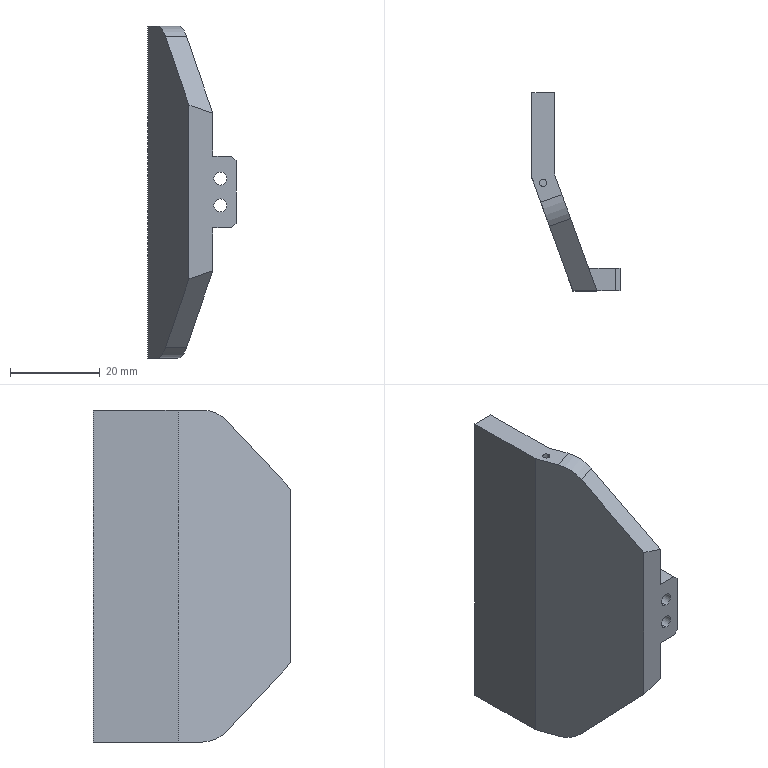Part | NX | 1 solid | 38 faces | box 19.643 x 44.061 x 74 mm | volume 15550 mm3 | plane 20 | cylinder 10 | cone 8 | commonest cylinder face diameters 1.6 x4 2.9 x4 16 x2
STEP:
#1=CARTESIAN_POINT('',(-19.643,44.061,-74.));
#2=VERTEX_POINT('',#1);
#3=CARTESIAN_POINT('',(-19.643,44.061,0.));
#4=VERTEX_POINT('',#3);
#5=CARTESIAN_POINT('',(-19.643,44.061,-74.));
#6=DIRECTION('',(0.,0.,1.));
#7=VECTOR('',#6,1000.);
#8=LINE('',#5,#7);
#9=EDGE_CURVE('',#2,#4,#8,.T.);
#10=ORIENTED_EDGE('',*,*,#9,.F.);
#11=CARTESIAN_POINT('',(-19.643,25.118,-74.));
#12=VERTEX_POINT('',#11);
#13=CARTESIAN_POINT('',(-19.643,34.6,-74.));
#14=DIRECTION('',(0.,-1.,0.));
#15=VECTOR('',#14,1000.);
#16=LINE('',#13,#15);
#17=EDGE_CURVE('',#2,#12,#16,.T.);
#18=ORIENTED_EDGE('',*,*,#17,.T.);
#19=CARTESIAN_POINT('',(-19.643,25.118,0.));
#20=VERTEX_POINT('',#19);
#21=CARTESIAN_POINT('',(-19.643,25.118,-74.));
#22=DIRECTION('',(0.,0.,1.));
#23=VECTOR('',#22,1000.);
#24=LINE('',#21,#23);
#25=EDGE_CURVE('',#12,#20,#24,.T.);
#26=ORIENTED_EDGE('',*,*,#25,.T.);
#27=CARTESIAN_POINT('',(-19.643,34.6,0.));
#28=DIRECTION('',(0.,-1.,0.));
#29=VECTOR('',#28,1000.);
#30=LINE('',#27,#29);
#31=EDGE_CURVE('',#4,#20,#30,.T.);
#32=ORIENTED_EDGE('',*,*,#31,.F.);
#33=EDGE_LOOP('',(#10,#18,#26,#32));
#34=FACE_BOUND('',#33,.T.);
#35=CARTESIAN_POINT('',(-19.643,34.6,-74.));
#36=DIRECTION('',(-1.,0.,0.));
#37=DIRECTION('',(0.,0.,1.));
#38=AXIS2_PLACEMENT_3D('',#35,#36,#37);
#39=PLANE('',#38);
#40=ADVANCED_FACE('',(#34),#39,.T.);
#41=CARTESIAN_POINT('',(-14.643,26.,0.));
#42=VERTEX_POINT('',#41);
#43=CARTESIAN_POINT('',(-14.643,44.061,0.));
#44=VERTEX_POINT('',#43);
#45=CARTESIAN_POINT('',(-14.643,34.6,0.));
#46=DIRECTION('',(0.,1.,0.));
#47=VECTOR('',#46,1000.);
#48=LINE('',#45,#47);
#49=EDGE_CURVE('',#42,#44,#48,.T.);
#50=ORIENTED_EDGE('',*,*,#49,.T.);
#51=CARTESIAN_POINT('',(0.,44.061,0.));
#52=DIRECTION('',(-1.,0.,0.));
#53=VECTOR('',#52,1000.);
#54=LINE('',#51,#53);
#55=EDGE_CURVE('',#44,#4,#54,.T.);
#56=ORIENTED_EDGE('',*,*,#55,.T.);
#57=ORIENTED_EDGE('',*,*,#31,.T.);
#58=CARTESIAN_POINT('',(-17.662,19.674,0.));
#59=VERTEX_POINT('',#58);
#60=CARTESIAN_POINT('',(-10.501,0.,0.));
#61=DIRECTION('',(0.342,-0.9397,0.));
#62=VECTOR('',#61,1000.);
#63=LINE('',#60,#62);
#64=EDGE_CURVE('',#20,#59,#63,.T.);
#65=ORIENTED_EDGE('',*,*,#64,.T.);
#66=CARTESIAN_POINT('',(-12.963,21.384,0.));
#67=VERTEX_POINT('',#66);
#68=CARTESIAN_POINT('',(-12.963,21.384,0.));
#69=DIRECTION('',(0.9397,0.342,0.));
#70=VECTOR('',#69,1000.);
#71=LINE('',#68,#70);
#72=EDGE_CURVE('',#59,#67,#71,.T.);
#73=ORIENTED_EDGE('',*,*,#72,.T.);
#74=CARTESIAN_POINT('',(-14.643,26.,0.));
#75=DIRECTION('',(-0.342,0.9397,0.));
#76=VECTOR('',#75,1000.);
#77=LINE('',#74,#76);
#78=EDGE_CURVE('',#67,#42,#77,.T.);
#79=ORIENTED_EDGE('',*,*,#78,.T.);
#80=EDGE_LOOP('',(#50,#56,#57,#65,#73,#79));
#81=FACE_BOUND('',#80,.T.);
#82=CARTESIAN_POINT('',(-17.943,24.061,0.));
#83=VERTEX_POINT('',#82);
#84=CARTESIAN_POINT('',(-16.343,24.061,0.));
#85=VERTEX_POINT('',#84);
#86=CARTESIAN_POINT('',(-17.143,24.061,0.));
#87=DIRECTION('',(0.,0.,-1.));
#88=DIRECTION('',(-1.,0.,0.));
#89=AXIS2_PLACEMENT_3D('',#86,#87,#88);
#90=CIRCLE('',#89,0.8);
#91=EDGE_CURVE('',#83,#85,#90,.T.);
#92=ORIENTED_EDGE('',*,*,#91,.T.);
#93=CARTESIAN_POINT('',(-17.143,24.061,0.));
#94=DIRECTION('',(0.,0.,-1.));
#95=DIRECTION('',(-1.,0.,0.));
#96=AXIS2_PLACEMENT_3D('',#93,#94,#95);
#97=CIRCLE('',#96,0.8);
#98=EDGE_CURVE('',#85,#83,#97,.T.);
#99=ORIENTED_EDGE('',*,*,#98,.T.);
#100=EDGE_LOOP('',(#92,#99));
#101=FACE_BOUND('',#100,.T.);
#102=CARTESIAN_POINT('',(0.,0.,0.));
#103=DIRECTION('',(0.,0.,-1.));
#104=DIRECTION('',(-1.,0.,0.));
#105=AXIS2_PLACEMENT_3D('',#102,#103,#104);
#106=PLANE('',#105);
#107=ADVANCED_FACE('',(#81,#101),#106,.F.);
#108=CARTESIAN_POINT('',(-14.643,44.061,-74.));
#109=VERTEX_POINT('',#108);
#110=CARTESIAN_POINT('',(0.,44.061,-74.));
#111=DIRECTION('',(-1.,0.,0.));
#112=VECTOR('',#111,1000.);
#113=LINE('',#110,#112);
#114=EDGE_CURVE('',#109,#2,#113,.T.);
#115=ORIENTED_EDGE('',*,*,#114,.F.);
#116=CARTESIAN_POINT('',(-14.643,26.,-74.));
#117=VERTEX_POINT('',#116);
#118=CARTESIAN_POINT('',(-14.643,34.6,-74.));
#119=DIRECTION('',(0.,1.,0.));
#120=VECTOR('',#119,1000.);
#121=LINE('',#118,#120);
#122=EDGE_CURVE('',#117,#109,#121,.T.);
#123=ORIENTED_EDGE('',*,*,#122,.F.);
#124=CARTESIAN_POINT('',(-12.963,21.384,-74.));
#125=VERTEX_POINT('',#124);
#126=CARTESIAN_POINT('',(-14.643,26.,-74.));
#127=DIRECTION('',(-0.342,0.9397,0.));
#128=VECTOR('',#127,1000.);
#129=LINE('',#126,#128);
#130=EDGE_CURVE('',#125,#117,#129,.T.);
#131=ORIENTED_EDGE('',*,*,#130,.F.);
#132=CARTESIAN_POINT('',(-17.662,19.674,-74.));
#133=VERTEX_POINT('',#132);
#134=CARTESIAN_POINT('',(-17.662,19.674,-74.));
#135=DIRECTION('',(-0.9397,-0.342,0.));
#136=VECTOR('',#135,1000.);
#137=LINE('',#134,#136);
#138=EDGE_CURVE('',#125,#133,#137,.T.);
#139=ORIENTED_EDGE('',*,*,#138,.T.);
#140=CARTESIAN_POINT('',(-10.501,0.,-74.));
#141=DIRECTION('',(0.342,-0.9397,0.));
#142=VECTOR('',#141,1000.);
#143=LINE('',#140,#142);
#144=EDGE_CURVE('',#12,#133,#143,.T.);
#145=ORIENTED_EDGE('',*,*,#144,.F.);
#146=ORIENTED_EDGE('',*,*,#17,.F.);
#147=EDGE_LOOP('',(#115,#123,#131,#139,#145,#146));
#148=FACE_BOUND('',#147,.T.);
#149=CARTESIAN_POINT('',(-17.943,24.061,-74.));
#150=VERTEX_POINT('',#149);
#151=CARTESIAN_POINT('',(-16.343,24.061,-74.));
#152=VERTEX_POINT('',#151);
#153=CARTESIAN_POINT('',(-17.143,24.061,-74.));
#154=DIRECTION('',(0.,0.,-1.));
#155=DIRECTION('',(-1.,0.,0.));
#156=AXIS2_PLACEMENT_3D('',#153,#154,#155);
#157=CIRCLE('',#156,0.8);
#158=EDGE_CURVE('',#150,#152,#157,.T.);
#159=ORIENTED_EDGE('',*,*,#158,.F.);
#160=CARTESIAN_POINT('',(-17.143,24.061,-74.));
#161=DIRECTION('',(0.,0.,-1.));
#162=DIRECTION('',(-1.,0.,0.));
#163=AXIS2_PLACEMENT_3D('',#160,#161,#162);
#164=CIRCLE('',#163,0.8);
#165=EDGE_CURVE('',#152,#150,#164,.T.);
#166=ORIENTED_EDGE('',*,*,#165,.F.);
#167=EDGE_LOOP('',(#159,#166));
#168=FACE_BOUND('',#167,.T.);
#169=CARTESIAN_POINT('',(0.,0.,-74.));
#170=DIRECTION('',(0.,0.,-1.));
#171=DIRECTION('',(-1.,0.,0.));
#172=AXIS2_PLACEMENT_3D('',#169,#170,#171);
#173=PLANE('',#172);
#174=ADVANCED_FACE('',(#148,#168),#173,.T.);
#175=CARTESIAN_POINT('',(-17.943,24.061,-5.));
#176=VERTEX_POINT('',#175);
#177=CARTESIAN_POINT('',(-17.943,24.061,-74.));
#178=DIRECTION('',(0.,0.,-1.));
#179=VECTOR('',#178,1000.);
#180=LINE('',#177,#179);
#181=EDGE_CURVE('',#176,#83,#180,.F.);
#182=ORIENTED_EDGE('',*,*,#181,.F.);
#183=CARTESIAN_POINT('',(-16.343,24.061,-5.));
#184=VERTEX_POINT('',#183);
#185=CARTESIAN_POINT('',(-17.143,24.061,-5.));
#186=DIRECTION('',(0.,0.,1.));
#187=DIRECTION('',(1.,0.,0.));
#188=AXIS2_PLACEMENT_3D('',#185,#186,#187);
#189=CIRCLE('',#188,0.8);
#190=EDGE_CURVE('',#176,#184,#189,.F.);
#191=ORIENTED_EDGE('',*,*,#190,.T.);
#192=CARTESIAN_POINT('',(-16.343,24.061,-74.));
#193=DIRECTION('',(0.,0.,-1.));
#194=VECTOR('',#193,1000.);
#195=LINE('',#192,#194);
#196=EDGE_CURVE('',#184,#85,#195,.F.);
#197=ORIENTED_EDGE('',*,*,#196,.T.);
#198=ORIENTED_EDGE('',*,*,#91,.F.);
#199=EDGE_LOOP('',(#182,#191,#197,#198));
#200=FACE_BOUND('',#199,.T.);
#201=CARTESIAN_POINT('',(-17.143,24.061,-74.));
#202=DIRECTION('',(0.,0.,-1.));
#203=DIRECTION('',(-1.,0.,0.));
#204=AXIS2_PLACEMENT_3D('',#201,#202,#203);
#205=CYLINDRICAL_SURFACE('',#204,0.8);
#206=ADVANCED_FACE('',(#200),#205,.F.);
#207=CARTESIAN_POINT('',(-16.343,24.061,-68.));
#208=VERTEX_POINT('',#207);
#209=CARTESIAN_POINT('',(-16.343,24.061,-74.));
#210=DIRECTION('',(0.,0.,-1.));
#211=VECTOR('',#210,1000.);
#212=LINE('',#209,#211);
#213=EDGE_CURVE('',#152,#208,#212,.F.);
#214=ORIENTED_EDGE('',*,*,#213,.T.);
#215=CARTESIAN_POINT('',(-17.943,24.061,-68.));
#216=VERTEX_POINT('',#215);
#217=CARTESIAN_POINT('',(-17.143,24.061,-68.));
#218=DIRECTION('',(0.,0.,1.));
#219=DIRECTION('',(1.,0.,0.));
#220=AXIS2_PLACEMENT_3D('',#217,#218,#219);
#221=CIRCLE('',#220,0.8);
#222=EDGE_CURVE('',#208,#216,#221,.T.);
#223=ORIENTED_EDGE('',*,*,#222,.T.);
#224=CARTESIAN_POINT('',(-17.943,24.061,-74.));
#225=DIRECTION('',(0.,0.,-1.));
#226=VECTOR('',#225,1000.);
#227=LINE('',#224,#226);
#228=EDGE_CURVE('',#150,#216,#227,.F.);
#229=ORIENTED_EDGE('',*,*,#228,.F.);
#230=ORIENTED_EDGE('',*,*,#158,.T.);
#231=EDGE_LOOP('',(#214,#223,#229,#230));
#232=FACE_BOUND('',#231,.T.);
#233=CARTESIAN_POINT('',(-17.143,24.061,-74.));
#234=DIRECTION('',(0.,0.,-1.));
#235=DIRECTION('',(-1.,0.,0.));
#236=AXIS2_PLACEMENT_3D('',#233,#234,#235);
#237=CYLINDRICAL_SURFACE('',#236,0.8);
#238=ADVANCED_FACE('',(#232),#237,.F.);
#239=CARTESIAN_POINT('',(0.,0.,-30.));
#240=VERTEX_POINT('',#239);
#241=CARTESIAN_POINT('',(-1.,0.,-29.));
#242=VERTEX_POINT('',#241);
#243=CARTESIAN_POINT('',(22.,0.,-52.));
#244=DIRECTION('',(-0.7071,0.,0.7071));
#245=VECTOR('',#244,1000.);
#246=LINE('',#243,#245);
#247=EDGE_CURVE('',#240,#242,#246,.T.);
#248=ORIENTED_EDGE('',*,*,#247,.F.);
#249=CARTESIAN_POINT('',(0.,5.,-30.));
#250=VERTEX_POINT('',#249);
#251=CARTESIAN_POINT('',(0.,5.,-30.));
#252=DIRECTION('',(0.,-1.,0.));
#253=VECTOR('',#252,1000.);
#254=LINE('',#251,#253);
#255=EDGE_CURVE('',#250,#240,#254,.T.);
#256=ORIENTED_EDGE('',*,*,#255,.F.);
#257=CARTESIAN_POINT('',(-1.,5.,-29.));
#258=VERTEX_POINT('',#257);
#259=CARTESIAN_POINT('',(18.5,5.,-48.5));
#260=DIRECTION('',(0.7071,0.,-0.7071));
#261=VECTOR('',#260,1000.);
#262=LINE('',#259,#261);
#263=EDGE_CURVE('',#258,#250,#262,.T.);
#264=ORIENTED_EDGE('',*,*,#263,.F.);
#265=CARTESIAN_POINT('',(-1.,4.336,-29.));
#266=DIRECTION('',(0.,1.,0.));
#267=VECTOR('',#266,1000.);
#268=LINE('',#265,#267);
#269=EDGE_CURVE('',#242,#258,#268,.T.);
#270=ORIENTED_EDGE('',*,*,#269,.F.);
#271=EDGE_LOOP('',(#248,#256,#264,#270));
#272=FACE_BOUND('',#271,.T.);
#273=CARTESIAN_POINT('',(-1.,4.336,-29.));
#274=DIRECTION('',(-0.7071,0.,-0.7071));
#275=DIRECTION('',(0.,1.,0.));
#276=AXIS2_PLACEMENT_3D('',#273,#274,#275);
#277=PLANE('',#276);
#278=ADVANCED_FACE('',(#272),#277,.F.);
#279=CARTESIAN_POINT('',(0.,5.,-44.));
#280=VERTEX_POINT('',#279);
#281=CARTESIAN_POINT('',(-1.,5.,-45.));
#282=VERTEX_POINT('',#281);
#283=CARTESIAN_POINT('',(-18.5,5.,-62.5));
#284=DIRECTION('',(-0.7071,0.,-0.7071));
#285=VECTOR('',#284,1000.);
#286=LINE('',#283,#285);
#287=EDGE_CURVE('',#280,#282,#286,.T.);
#288=ORIENTED_EDGE('',*,*,#287,.F.);
#289=CARTESIAN_POINT('',(0.,0.,-44.));
#290=VERTEX_POINT('',#289);
#291=CARTESIAN_POINT('',(0.,5.,-44.));
#292=DIRECTION('',(0.,1.,0.));
#293=VECTOR('',#292,1000.);
#294=LINE('',#291,#293);
#295=EDGE_CURVE('',#290,#280,#294,.T.);
#296=ORIENTED_EDGE('',*,*,#295,.F.);
#297=CARTESIAN_POINT('',(-1.,0.,-45.));
#298=VERTEX_POINT('',#297);
#299=CARTESIAN_POINT('',(-15.,0.,-59.));
#300=DIRECTION('',(0.7071,0.,0.7071));
#301=VECTOR('',#300,1000.);
#302=LINE('',#299,#301);
#303=EDGE_CURVE('',#298,#290,#302,.T.);
#304=ORIENTED_EDGE('',*,*,#303,.F.);
#305=CARTESIAN_POINT('',(-1.,18.819,-45.));
#306=DIRECTION('',(0.,-1.,0.));
#307=VECTOR('',#306,1000.);
#308=LINE('',#305,#307);
#309=EDGE_CURVE('',#282,#298,#308,.T.);
#310=ORIENTED_EDGE('',*,*,#309,.F.);
#311=EDGE_LOOP('',(#288,#296,#304,#310));
#312=FACE_BOUND('',#311,.T.);
#313=CARTESIAN_POINT('',(-1.,18.819,-45.));
#314=DIRECTION('',(-0.7071,0.,0.7071));
#315=DIRECTION('',(0.,-1.,0.));
#316=AXIS2_PLACEMENT_3D('',#313,#314,#315);
#317=PLANE('',#316);
#318=ADVANCED_FACE('',(#312),#317,.F.);
#319=CARTESIAN_POINT('',(-3.5,3.7,-35.45));
#320=VERTEX_POINT('',#319);
#321=CARTESIAN_POINT('',(-3.5,5.,-36.75));
#322=VERTEX_POINT('',#321);
#323=CARTESIAN_POINT('',(-3.5,5.,-36.75));
#324=DIRECTION('',(0.,0.7071,-0.7071));
#325=VECTOR('',#324,1000.);
#326=LINE('',#323,#325);
#327=EDGE_CURVE('',#320,#322,#326,.T.);
#328=ORIENTED_EDGE('',*,*,#327,.F.);
#329=CARTESIAN_POINT('',(-3.5,3.7,-32.55));
#330=VERTEX_POINT('',#329);
#331=CARTESIAN_POINT('',(-3.5,3.7,-34.));
#332=DIRECTION('',(0.,1.,0.));
#333=DIRECTION('',(0.,0.,1.));
#334=AXIS2_PLACEMENT_3D('',#331,#332,#333);
#335=CIRCLE('',#334,1.45);
#336=EDGE_CURVE('',#330,#320,#335,.T.);
#337=ORIENTED_EDGE('',*,*,#336,.F.);
#338=CARTESIAN_POINT('',(-3.5,5.,-31.25));
#339=VERTEX_POINT('',#338);
#340=CARTESIAN_POINT('',(-3.5,5.,-31.25));
#341=DIRECTION('',(0.,0.7071,0.7071));
#342=VECTOR('',#341,1000.);
#343=LINE('',#340,#342);
#344=EDGE_CURVE('',#330,#339,#343,.T.);
#345=ORIENTED_EDGE('',*,*,#344,.T.);
#346=CARTESIAN_POINT('',(-3.5,5.,-34.));
#347=DIRECTION('',(0.,1.,0.));
#348=DIRECTION('',(0.,0.,1.));
#349=AXIS2_PLACEMENT_3D('',#346,#347,#348);
#350=CIRCLE('',#349,2.75);
#351=EDGE_CURVE('',#339,#322,#350,.T.);
#352=ORIENTED_EDGE('',*,*,#351,.T.);
#353=EDGE_LOOP('',(#328,#337,#345,#352));
#354=FACE_BOUND('',#353,.T.);
#355=CARTESIAN_POINT('',(-3.5,5.,-34.));
#356=DIRECTION('',(0.,1.,0.));
#357=DIRECTION('',(0.,0.,1.));
#358=AXIS2_PLACEMENT_3D('',#355,#356,#357);
#359=CONICAL_SURFACE('',#358,2.75,0.7854);
#360=ADVANCED_FACE('',(#354),#359,.F.);
#361=CARTESIAN_POINT('',(-3.5,0.,-35.45));
#362=VERTEX_POINT('',#361);
#363=CARTESIAN_POINT('',(-3.5,5.,-35.45));
#364=DIRECTION('',(0.,1.,0.));
#365=VECTOR('',#364,1000.);
#366=LINE('',#363,#365);
#367=EDGE_CURVE('',#362,#320,#366,.T.);
#368=ORIENTED_EDGE('',*,*,#367,.F.);
#369=CARTESIAN_POINT('',(-3.5,0.,-32.55));
#370=VERTEX_POINT('',#369);
#371=CARTESIAN_POINT('',(-3.5,0.,-34.));
#372=DIRECTION('',(0.,-1.,0.));
#373=DIRECTION('',(1.,0.,0.));
#374=AXIS2_PLACEMENT_3D('',#371,#372,#373);
#375=CIRCLE('',#374,1.45);
#376=EDGE_CURVE('',#362,#370,#375,.T.);
#377=ORIENTED_EDGE('',*,*,#376,.T.);
#378=CARTESIAN_POINT('',(-3.5,5.,-32.55));
#379=DIRECTION('',(0.,1.,0.));
#380=VECTOR('',#379,1000.);
#381=LINE('',#378,#380);
#382=EDGE_CURVE('',#370,#330,#381,.T.);
#383=ORIENTED_EDGE('',*,*,#382,.T.);
#384=ORIENTED_EDGE('',*,*,#336,.T.);
#385=EDGE_LOOP('',(#368,#377,#383,#384));
#386=FACE_BOUND('',#385,.T.);
#387=CARTESIAN_POINT('',(-3.5,5.,-34.));
#388=DIRECTION('',(0.,1.,0.));
#389=DIRECTION('',(0.,0.,1.));
#390=AXIS2_PLACEMENT_3D('',#387,#388,#389);
#391=CYLINDRICAL_SURFACE('',#390,1.45);
#392=ADVANCED_FACE('',(#386),#391,.F.);
#393=CARTESIAN_POINT('',(-3.5,3.7,-41.45));
#394=VERTEX_POINT('',#393);
#395=CARTESIAN_POINT('',(-3.5,5.,-42.75));
#396=VERTEX_POINT('',#395);
#397=CARTESIAN_POINT('',(-3.5,5.,-42.75));
#398=DIRECTION('',(0.,0.7071,-0.7071));
#399=VECTOR('',#398,1000.);
#400=LINE('',#397,#399);
#401=EDGE_CURVE('',#394,#396,#400,.T.);
#402=ORIENTED_EDGE('',*,*,#401,.F.);
#403=CARTESIAN_POINT('',(-3.5,3.7,-38.55));
#404=VERTEX_POINT('',#403);
#405=CARTESIAN_POINT('',(-3.5,3.7,-40.));
#406=DIRECTION('',(0.,1.,0.));
#407=DIRECTION('',(0.,0.,1.));
#408=AXIS2_PLACEMENT_3D('',#405,#406,#407);
#409=CIRCLE('',#408,1.45);
#410=EDGE_CURVE('',#404,#394,#409,.T.);
#411=ORIENTED_EDGE('',*,*,#410,.F.);
#412=CARTESIAN_POINT('',(-3.5,5.,-37.25));
#413=VERTEX_POINT('',#412);
#414=CARTESIAN_POINT('',(-3.5,5.,-37.25));
#415=DIRECTION('',(0.,0.7071,0.7071));
#416=VECTOR('',#415,1000.);
#417=LINE('',#414,#416);
#418=EDGE_CURVE('',#404,#413,#417,.T.);
#419=ORIENTED_EDGE('',*,*,#418,.T.);
#420=CARTESIAN_POINT('',(-3.5,5.,-40.));
#421=DIRECTION('',(0.,1.,0.));
#422=DIRECTION('',(0.,0.,1.));
#423=AXIS2_PLACEMENT_3D('',#420,#421,#422);
#424=CIRCLE('',#423,2.75);
#425=EDGE_CURVE('',#413,#396,#424,.T.);
#426=ORIENTED_EDGE('',*,*,#425,.T.);
#427=EDGE_LOOP('',(#402,#411,#419,#426));
#428=FACE_BOUND('',#427,.T.);
#429=CARTESIAN_POINT('',(-3.5,5.,-40.));
#430=DIRECTION('',(0.,1.,0.));
#431=DIRECTION('',(0.,0.,1.));
#432=AXIS2_PLACEMENT_3D('',#429,#430,#431);
#433=CONICAL_SURFACE('',#432,2.75,0.7854);
#434=ADVANCED_FACE('',(#428),#433,.F.);
#435=CARTESIAN_POINT('',(-3.5,0.,-41.45));
#436=VERTEX_POINT('',#435);
#437=CARTESIAN_POINT('',(-3.5,5.,-41.45));
#438=DIRECTION('',(0.,1.,0.));
#439=VECTOR('',#438,1000.);
#440=LINE('',#437,#439);
#441=EDGE_CURVE('',#436,#394,#440,.T.);
#442=ORIENTED_EDGE('',*,*,#441,.F.);
#443=CARTESIAN_POINT('',(-3.5,0.,-38.55));
#444=VERTEX_POINT('',#443);
#445=CARTESIAN_POINT('',(-3.5,0.,-40.));
#446=DIRECTION('',(0.,-1.,0.));
#447=DIRECTION('',(1.,0.,0.));
#448=AXIS2_PLACEMENT_3D('',#445,#446,#447);
#449=CIRCLE('',#448,1.45);
#450=EDGE_CURVE('',#436,#444,#449,.T.);
#451=ORIENTED_EDGE('',*,*,#450,.T.);
#452=CARTESIAN_POINT('',(-3.5,5.,-38.55));
#453=DIRECTION('',(0.,1.,0.));
#454=VECTOR('',#453,1000.);
#455=LINE('',#452,#454);
#456=EDGE_CURVE('',#444,#404,#455,.T.);
#457=ORIENTED_EDGE('',*,*,#456,.T.);
#458=ORIENTED_EDGE('',*,*,#410,.T.);
#459=EDGE_LOOP('',(#442,#451,#457,#458));
#460=FACE_BOUND('',#459,.T.);
#461=CARTESIAN_POINT('',(-3.5,5.,-40.));
#462=DIRECTION('',(0.,1.,0.));
#463=DIRECTION('',(0.,0.,1.));
#464=AXIS2_PLACEMENT_3D('',#461,#462,#463);
#465=CYLINDRICAL_SURFACE('',#464,1.45);
#466=ADVANCED_FACE('',(#460),#465,.F.);
#467=CARTESIAN_POINT('',(-7.,5.,-45.));
#468=VERTEX_POINT('',#467);
#469=CARTESIAN_POINT('',(6.641,5.,-45.));
#470=DIRECTION('',(1.,0.,0.));
#471=VECTOR('',#470,1000.);
#472=LINE('',#469,#471);
#473=EDGE_CURVE('',#468,#282,#472,.T.);
#474=ORIENTED_EDGE('',*,*,#473,.T.);
#475=ORIENTED_EDGE('',*,*,#309,.T.);
#476=CARTESIAN_POINT('',(-5.18,0.,-45.));
#477=VERTEX_POINT('',#476);
#478=CARTESIAN_POINT('',(6.641,0.,-45.));
#479=DIRECTION('',(-1.,0.,0.));
#480=VECTOR('',#479,1000.);
#481=LINE('',#478,#480);
#482=EDGE_CURVE('',#298,#477,#481,.T.);
#483=ORIENTED_EDGE('',*,*,#482,.T.);
#484=CARTESIAN_POINT('',(-9.846,12.819,-45.));
#485=DIRECTION('',(0.342,-0.9397,0.));
#486=VECTOR('',#485,1000.);
#487=LINE('',#484,#486);
#488=EDGE_CURVE('',#468,#477,#487,.T.);
#489=ORIENTED_EDGE('',*,*,#488,.F.);
#490=EDGE_LOOP('',(#474,#475,#483,#489));
#491=FACE_BOUND('',#490,.T.);
#492=CARTESIAN_POINT('',(6.641,18.819,-45.));
#493=DIRECTION('',(0.,0.,-1.));
#494=DIRECTION('',(-1.,0.,0.));
#495=AXIS2_PLACEMENT_3D('',#492,#493,#494);
#496=PLANE('',#495);
#497=ADVANCED_FACE('',(#491),#496,.T.);
#498=CARTESIAN_POINT('',(-5.18,0.,-29.));
#499=VERTEX_POINT('',#498);
#500=CARTESIAN_POINT('',(11.912,0.,-29.));
#501=DIRECTION('',(1.,0.,0.));
#502=VECTOR('',#501,1000.);
#503=LINE('',#500,#502);
#504=EDGE_CURVE('',#499,#242,#503,.T.);
#505=ORIENTED_EDGE('',*,*,#504,.T.);
#506=ORIENTED_EDGE('',*,*,#269,.T.);
#507=CARTESIAN_POINT('',(-7.,5.,-29.));
#508=VERTEX_POINT('',#507);
#509=CARTESIAN_POINT('',(11.912,5.,-29.));
#510=DIRECTION('',(-1.,0.,0.));
#511=VECTOR('',#510,1000.);
#512=LINE('',#509,#511);
#513=EDGE_CURVE('',#258,#508,#512,.T.);
#514=ORIENTED_EDGE('',*,*,#513,.T.);
#515=CARTESIAN_POINT('',(-4.574,-1.665,-29.));
#516=DIRECTION('',(-0.342,0.9397,0.));
#517=VECTOR('',#516,1000.);
#518=LINE('',#515,#517);
#519=EDGE_CURVE('',#499,#508,#518,.T.);
#520=ORIENTED_EDGE('',*,*,#519,.F.);
#521=EDGE_LOOP('',(#505,#506,#514,#520));
#522=FACE_BOUND('',#521,.T.);
#523=CARTESIAN_POINT('',(11.912,4.336,-29.));
#524=DIRECTION('',(0.,0.,1.));
#525=DIRECTION('',(1.,0.,0.));
#526=AXIS2_PLACEMENT_3D('',#523,#524,#525);
#527=PLANE('',#526);
#528=ADVANCED_FACE('',(#522),#527,.T.);
#529=CARTESIAN_POINT('',(-15.727,14.359,-71.657));
#530=VERTEX_POINT('',#529);
#531=CARTESIAN_POINT('',(-17.662,19.674,-66.));
#532=DIRECTION('',(-0.9397,-0.342,0.));
#533=DIRECTION('',(0.342,-0.9397,0.));
#534=AXIS2_PLACEMENT_3D('',#531,#532,#533);
#535=CIRCLE('',#534,8.);
#536=EDGE_CURVE('',#133,#530,#535,.T.);
#537=ORIENTED_EDGE('',*,*,#536,.F.);
#538=ORIENTED_EDGE('',*,*,#138,.F.);
#539=CARTESIAN_POINT('',(-11.029,16.069,-71.657));
#540=VERTEX_POINT('',#539);
#541=CARTESIAN_POINT('',(-12.963,21.384,-66.));
#542=DIRECTION('',(0.9397,0.342,0.));
#543=DIRECTION('',(-0.342,0.9397,0.));
#544=AXIS2_PLACEMENT_3D('',#541,#542,#543);
#545=CIRCLE('',#544,8.);
#546=EDGE_CURVE('',#540,#125,#545,.T.);
#547=ORIENTED_EDGE('',*,*,#546,.F.);
#548=CARTESIAN_POINT('',(-11.029,16.069,-71.657));
#549=DIRECTION('',(0.9397,0.342,0.));
#550=VECTOR('',#549,1000.);
#551=LINE('',#548,#550);
#552=EDGE_CURVE('',#530,#540,#551,.T.);
#553=ORIENTED_EDGE('',*,*,#552,.F.);
#554=EDGE_LOOP('',(#537,#538,#547,#553));
#555=FACE_BOUND('',#554,.T.);
#556=CARTESIAN_POINT('',(-25.735,16.736,-66.));
#557=DIRECTION('',(-0.9397,-0.342,0.));
#558=DIRECTION('',(0.342,-0.9397,0.));
#559=AXIS2_PLACEMENT_3D('',#556,#557,#558);
#560=CYLINDRICAL_SURFACE('',#559,8.);
#561=ADVANCED_FACE('',(#555),#560,.T.);
#562=CARTESIAN_POINT('',(-11.029,16.069,-2.343));
#563=VERTEX_POINT('',#562);
#564=CARTESIAN_POINT('',(-12.963,21.384,-8.));
#565=DIRECTION('',(0.9397,0.342,0.));
#566=DIRECTION('',(-0.342,0.9397,0.));
#567=AXIS2_PLACEMENT_3D('',#564,#565,#566);
#568=CIRCLE('',#567,8.);
#569=EDGE_CURVE('',#67,#563,#568,.T.);
#570=ORIENTED_EDGE('',*,*,#569,.F.);
#571=ORIENTED_EDGE('',*,*,#72,.F.);
#572=CARTESIAN_POINT('',(-15.727,14.359,-2.343));
#573=VERTEX_POINT('',#572);
#574=CARTESIAN_POINT('',(-17.662,19.674,-8.));
#575=DIRECTION('',(-0.9397,-0.342,0.));
#576=DIRECTION('',(0.342,-0.9397,0.));
#577=AXIS2_PLACEMENT_3D('',#574,#575,#576);
#578=CIRCLE('',#577,8.);
#579=EDGE_CURVE('',#573,#59,#578,.T.);
#580=ORIENTED_EDGE('',*,*,#579,.F.);
#581=CARTESIAN_POINT('',(-15.727,14.359,-2.343));
#582=DIRECTION('',(-0.9397,-0.342,0.));
#583=VECTOR('',#582,1000.);
#584=LINE('',#581,#583);
#585=EDGE_CURVE('',#563,#573,#584,.T.);
#586=ORIENTED_EDGE('',*,*,#585,.F.);
#587=EDGE_LOOP('',(#570,#571,#580,#586));
#588=FACE_BOUND('',#587,.T.);
#589=CARTESIAN_POINT('',(-25.735,16.736,-8.));
#590=DIRECTION('',(0.9397,0.342,0.));
#591=DIRECTION('',(-0.342,0.9397,0.));
#592=AXIS2_PLACEMENT_3D('',#589,#590,#591);
#593=CYLINDRICAL_SURFACE('',#592,8.);
#594=ADVANCED_FACE('',(#588),#593,.T.);
#595=CARTESIAN_POINT('',(-7.,5.,-74.));
#596=DIRECTION('',(0.,0.,-1.));
#597=VECTOR('',#596,1000.);
#598=LINE('',#595,#597);
#599=EDGE_CURVE('',#508,#468,#598,.T.);
#600=ORIENTED_EDGE('',*,*,#599,.T.);
#601=ORIENTED_EDGE('',*,*,#488,.T.);
#602=CARTESIAN_POINT('',(-5.18,0.,-54.557));
#603=VERTEX_POINT('',#602);
#604=CARTESIAN_POINT('',(-5.18,0.,0.));
#605=DIRECTION('',(0.,0.,-1.));
#606=VECTOR('',#605,1000.);
#607=LINE('',#604,#606);
#608=EDGE_CURVE('',#477,#603,#607,.T.);
#609=ORIENTED_EDGE('',*,*,#608,.T.);
#610=CARTESIAN_POINT('',(-13.237,22.135,-78.113));
#611=DIRECTION('',(0.2418,-0.6645,0.7071));
#612=VECTOR('',#611,1000.);
#613=LINE('',#610,#612);
#614=EDGE_CURVE('',#540,#603,#613,.T.);
#615=ORIENTED_EDGE('',*,*,#614,.F.);
#616=ORIENTED_EDGE('',*,*,#546,.T.);
#617=ORIENTED_EDGE('',*,*,#130,.T.);
#618=CARTESIAN_POINT('',(-14.643,26.,-74.));
#619=DIRECTION('',(0.,0.,1.));
#620=VECTOR('',#619,1000.);
#621=LINE('',#618,#620);
#622=EDGE_CURVE('',#117,#42,#621,.T.);
#623=ORIENTED_EDGE('',*,*,#622,.T.);
#624=ORIENTED_EDGE('',*,*,#78,.F.);
#625=ORIENTED_EDGE('',*,*,#569,.T.);
#626=CARTESIAN_POINT('',(-5.18,0.,-19.443));
#627=VERTEX_POINT('',#626);
#628=CARTESIAN_POINT('',(-0.582,-12.633,-32.887));
#629=DIRECTION('',(0.2418,-0.6645,-0.7071));
#630=VECTOR('',#629,1000.);
#631=LINE('',#628,#630);
#632=EDGE_CURVE('',#563,#627,#631,.T.);
#633=ORIENTED_EDGE('',*,*,#632,.T.);
#634=CARTESIAN_POINT('',(-5.18,0.,0.));
#635=DIRECTION('',(0.,0.,-1.));
#636=VECTOR('',#635,1000.);
#637=LINE('',#634,#636);
#638=EDGE_CURVE('',#627,#499,#637,.T.);
#639=ORIENTED_EDGE('',*,*,#638,.T.);
#640=ORIENTED_EDGE('',*,*,#519,.T.);
#641=EDGE_LOOP('',(#600,#601,#609,#615,#616,#617,#623,#624,#625,#633,#639,#640));
#642=FACE_BOUND('',#641,.T.);
#643=CARTESIAN_POINT('',(-14.643,26.,-74.));
#644=DIRECTION('',(0.9397,0.342,0.));
#645=DIRECTION('',(-0.342,0.9397,0.));
#646=AXIS2_PLACEMENT_3D('',#643,#644,#645);
#647=PLANE('',#646);
#648=ADVANCED_FACE('',(#642),#647,.T.);
#649=ORIENTED_EDGE('',*,*,#122,.T.);
#650=CARTESIAN_POINT('',(-14.643,44.061,-37.));
#651=DIRECTION('',(0.,0.,-1.));
#652=VECTOR('',#651,1000.);
#653=LINE('',#650,#652);
#654=EDGE_CURVE('',#44,#109,#653,.T.);
#655=ORIENTED_EDGE('',*,*,#654,.F.);
#656=ORIENTED_EDGE('',*,*,#49,.F.);
#657=ORIENTED_EDGE('',*,*,#622,.F.);
#658=EDGE_LOOP('',(#649,#655,#656,#657));
#659=FACE_BOUND('',#658,.T.);
#660=CARTESIAN_POINT('',(-14.643,34.6,-74.));
#661=DIRECTION('',(1.,0.,0.));
#662=DIRECTION('',(0.,1.,0.));
#663=AXIS2_PLACEMENT_3D('',#660,#661,#662);
#664=PLANE('',#663);
#665=ADVANCED_FACE('',(#659),#664,.T.);
#666=ORIENTED_EDGE('',*,*,#614,.T.);
#667=CARTESIAN_POINT('',(-10.501,0.,-56.377));
#668=VERTEX_POINT('',#667);
#669=CARTESIAN_POINT('',(-6.496,0.,-55.007));
#670=DIRECTION('',(-0.9462,0.,-0.3236));
#671=VECTOR('',#670,1000.);
#672=LINE('',#669,#671);
#673=EDGE_CURVE('',#603,#668,#672,.T.);
#674=ORIENTED_EDGE('',*,*,#673,.T.);
#675=CARTESIAN_POINT('',(-13.515,8.28,-65.188));
#676=DIRECTION('',(-0.2418,0.6645,-0.7071));
#677=VECTOR('',#676,1000.);
#678=LINE('',#675,#677);
#679=EDGE_CURVE('',#668,#530,#678,.T.);
#680=ORIENTED_EDGE('',*,*,#679,.T.);
#681=ORIENTED_EDGE('',*,*,#552,.T.);
#682=EDGE_LOOP('',(#666,#674,#680,#681));
#683=FACE_BOUND('',#682,.T.);
#684=CARTESIAN_POINT('',(-25.627,16.441,-77.));
#685=DIRECTION('',(-0.2418,0.6645,0.7071));
#686=DIRECTION('',(0.,-0.7287,0.6848));
#687=AXIS2_PLACEMENT_3D('',#684,#685,#686);
#688=PLANE('',#687);
#689=ADVANCED_FACE('',(#683),#688,.F.);
#690=CARTESIAN_POINT('',(-10.501,0.,-17.623));
#691=VERTEX_POINT('',#690);
#692=CARTESIAN_POINT('',(16.163,0.,-26.743));
#693=DIRECTION('',(-0.9462,0.,0.3236));
#694=VECTOR('',#693,1000.);
#695=LINE('',#692,#694);
#696=EDGE_CURVE('',#627,#691,#695,.T.);
#697=ORIENTED_EDGE('',*,*,#696,.F.);
#698=ORIENTED_EDGE('',*,*,#632,.F.);
#699=ORIENTED_EDGE('',*,*,#585,.T.);
#700=CARTESIAN_POINT('',(-0.86,-26.488,-45.812));
#701=DIRECTION('',(-0.2418,0.6645,0.7071));
#702=VECTOR('',#701,1000.);
#703=LINE('',#700,#702);
#704=EDGE_CURVE('',#691,#573,#703,.T.);
#705=ORIENTED_EDGE('',*,*,#704,.F.);
#706=EDGE_LOOP('',(#697,#698,#699,#705));
#707=FACE_BOUND('',#706,.T.);
#708=CARTESIAN_POINT('',(-25.627,16.441,3.));
#709=DIRECTION('',(0.2418,-0.6645,0.7071));
#710=DIRECTION('',(0.,-0.7287,-0.6848));
#711=AXIS2_PLACEMENT_3D('',#708,#709,#710);
#712=PLANE('',#711);
#713=ADVANCED_FACE('',(#707),#712,.T.);
#714=CARTESIAN_POINT('',(-10.501,0.,-74.));
#715=DIRECTION('',(0.,0.,1.));
#716=VECTOR('',#715,1000.);
#717=LINE('',#714,#716);
#718=EDGE_CURVE('',#668,#691,#717,.T.);
#719=ORIENTED_EDGE('',*,*,#718,.F.);
#720=ORIENTED_EDGE('',*,*,#673,.F.);
#721=ORIENTED_EDGE('',*,*,#608,.F.);
#722=ORIENTED_EDGE('',*,*,#482,.F.);
#723=ORIENTED_EDGE('',*,*,#303,.T.);
#724=CARTESIAN_POINT('',(0.,0.,-74.));
#725=DIRECTION('',(0.,0.,1.));
#726=VECTOR('',#725,1000.);
#727=LINE('',#724,#726);
#728=EDGE_CURVE('',#290,#240,#727,.T.);
#729=ORIENTED_EDGE('',*,*,#728,.T.);
#730=ORIENTED_EDGE('',*,*,#247,.T.);
#731=ORIENTED_EDGE('',*,*,#504,.F.);
#732=ORIENTED_EDGE('',*,*,#638,.F.);
#733=ORIENTED_EDGE('',*,*,#696,.T.);
#734=EDGE_LOOP('',(#719,#720,#721,#722,#723,#729,#730,#731,#732,#733));
#735=FACE_BOUND('',#734,.T.);
#736=CARTESIAN_POINT('',(-3.5,0.,-40.));
#737=DIRECTION('',(0.,-1.,0.));
#738=DIRECTION('',(1.,0.,0.));
#739=AXIS2_PLACEMENT_3D('',#736,#737,#738);
#740=CIRCLE('',#739,1.45);
#741=EDGE_CURVE('',#444,#436,#740,.T.);
#742=ORIENTED_EDGE('',*,*,#741,.F.);
#743=ORIENTED_EDGE('',*,*,#450,.F.);
#744=EDGE_LOOP('',(#742,#743));
#745=FACE_BOUND('',#744,.T.);
#746=CARTESIAN_POINT('',(-3.5,0.,-34.));
#747=DIRECTION('',(0.,-1.,0.));
#748=DIRECTION('',(1.,0.,0.));
#749=AXIS2_PLACEMENT_3D('',#746,#747,#748);
#750=CIRCLE('',#749,1.45);
#751=EDGE_CURVE('',#370,#362,#750,.T.);
#752=ORIENTED_EDGE('',*,*,#751,.F.);
#753=ORIENTED_EDGE('',*,*,#376,.F.);
#754=EDGE_LOOP('',(#752,#753));
#755=FACE_BOUND('',#754,.T.);
#756=CARTESIAN_POINT('',(0.,0.,-74.));
#757=DIRECTION('',(0.,-1.,0.));
#758=DIRECTION('',(1.,0.,0.));
#759=AXIS2_PLACEMENT_3D('',#756,#757,#758);
#760=PLANE('',#759);
#761=ADVANCED_FACE('',(#735,#745,#755),#760,.T.);
#762=ORIENTED_EDGE('',*,*,#728,.F.);
#763=ORIENTED_EDGE('',*,*,#295,.T.);
#764=CARTESIAN_POINT('',(0.,5.,-74.));
#765=DIRECTION('',(0.,0.,1.));
#766=VECTOR('',#765,1000.);
#767=LINE('',#764,#766);
#768=EDGE_CURVE('',#280,#250,#767,.T.);
#769=ORIENTED_EDGE('',*,*,#768,.T.);
#770=ORIENTED_EDGE('',*,*,#255,.T.);
#771=EDGE_LOOP('',(#762,#763,#769,#770));
#772=FACE_BOUND('',#771,.T.);
#773=CARTESIAN_POINT('',(0.,5.,-74.));
#774=DIRECTION('',(1.,0.,0.));
#775=DIRECTION('',(0.,0.,-1.));
#776=AXIS2_PLACEMENT_3D('',#773,#774,#775);
#777=PLANE('',#776);
#778=ADVANCED_FACE('',(#772),#777,.T.);
#779=ORIENTED_EDGE('',*,*,#768,.F.);
#780=ORIENTED_EDGE('',*,*,#287,.T.);
#781=ORIENTED_EDGE('',*,*,#473,.F.);
#782=ORIENTED_EDGE('',*,*,#599,.F.);
#783=ORIENTED_EDGE('',*,*,#513,.F.);
#784=ORIENTED_EDGE('',*,*,#263,.T.);
#785=EDGE_LOOP('',(#779,#780,#781,#782,#783,#784));
#786=FACE_BOUND('',#785,.T.);
#787=ORIENTED_EDGE('',*,*,#425,.F.);
#788=CARTESIAN_POINT('',(-3.5,5.,-40.));
#789=DIRECTION('',(0.,1.,0.));
#790=DIRECTION('',(0.,0.,1.));
#791=AXIS2_PLACEMENT_3D('',#788,#789,#790);
#792=CIRCLE('',#791,2.75);
#793=EDGE_CURVE('',#396,#413,#792,.T.);
#794=ORIENTED_EDGE('',*,*,#793,.F.);
#795=EDGE_LOOP('',(#787,#794));
#796=FACE_BOUND('',#795,.T.);
#797=ORIENTED_EDGE('',*,*,#351,.F.);
#798=CARTESIAN_POINT('',(-3.5,5.,-34.));
#799=DIRECTION('',(0.,1.,0.));
#800=DIRECTION('',(0.,0.,1.));
#801=AXIS2_PLACEMENT_3D('',#798,#799,#800);
#802=CIRCLE('',#801,2.75);
#803=EDGE_CURVE('',#322,#339,#802,.T.);
#804=ORIENTED_EDGE('',*,*,#803,.F.);
#805=EDGE_LOOP('',(#797,#804));
#806=FACE_BOUND('',#805,.T.);
#807=CARTESIAN_POINT('',(-7.,5.,-74.));
#808=DIRECTION('',(0.,1.,0.));
#809=DIRECTION('',(-1.,0.,0.));
#810=AXIS2_PLACEMENT_3D('',#807,#808,#809);
#811=PLANE('',#810);
#812=ADVANCED_FACE('',(#786,#796,#806),#811,.T.);
#813=ORIENTED_EDGE('',*,*,#679,.F.);
#814=ORIENTED_EDGE('',*,*,#718,.T.);
#815=ORIENTED_EDGE('',*,*,#704,.T.);
#816=ORIENTED_EDGE('',*,*,#579,.T.);
#817=ORIENTED_EDGE('',*,*,#64,.F.);
#818=ORIENTED_EDGE('',*,*,#25,.F.);
#819=ORIENTED_EDGE('',*,*,#144,.T.);
#820=ORIENTED_EDGE('',*,*,#536,.T.);
#821=EDGE_LOOP('',(#813,#814,#815,#816,#817,#818,#819,#820));
#822=FACE_BOUND('',#821,.T.);
#823=CARTESIAN_POINT('',(-10.501,0.,-74.));
#824=DIRECTION('',(-0.9397,-0.342,0.));
#825=DIRECTION('',(0.342,-0.9397,0.));
#826=AXIS2_PLACEMENT_3D('',#823,#824,#825);
#827=PLANE('',#826);
#828=ADVANCED_FACE('',(#822),#827,.T.);
#829=ORIENTED_EDGE('',*,*,#741,.T.);
#830=ORIENTED_EDGE('',*,*,#441,.T.);
#831=CARTESIAN_POINT('',(-3.5,3.7,-40.));
#832=DIRECTION('',(0.,1.,0.));
#833=DIRECTION('',(0.,0.,1.));
#834=AXIS2_PLACEMENT_3D('',#831,#832,#833);
#835=CIRCLE('',#834,1.45);
#836=EDGE_CURVE('',#394,#404,#835,.T.);
#837=ORIENTED_EDGE('',*,*,#836,.T.);
#838=ORIENTED_EDGE('',*,*,#456,.F.);
#839=EDGE_LOOP('',(#829,#830,#837,#838));
#840=FACE_BOUND('',#839,.T.);
#841=CARTESIAN_POINT('',(-3.5,5.,-40.));
#842=DIRECTION('',(0.,1.,0.));
#843=DIRECTION('',(0.,0.,1.));
#844=AXIS2_PLACEMENT_3D('',#841,#842,#843);
#845=CYLINDRICAL_SURFACE('',#844,1.45);
#846=ADVANCED_FACE('',(#840),#845,.F.);
#847=ORIENTED_EDGE('',*,*,#836,.F.);
#848=ORIENTED_EDGE('',*,*,#401,.T.);
#849=ORIENTED_EDGE('',*,*,#793,.T.);
#850=ORIENTED_EDGE('',*,*,#418,.F.);
#851=EDGE_LOOP('',(#847,#848,#849,#850));
#852=FACE_BOUND('',#851,.T.);
#853=CARTESIAN_POINT('',(-3.5,5.,-40.));
#854=DIRECTION('',(0.,1.,0.));
#855=DIRECTION('',(0.,0.,1.));
#856=AXIS2_PLACEMENT_3D('',#853,#854,#855);
#857=CONICAL_SURFACE('',#856,2.75,0.7854);
#858=ADVANCED_FACE('',(#852),#857,.F.);
#859=ORIENTED_EDGE('',*,*,#751,.T.);
#860=ORIENTED_EDGE('',*,*,#367,.T.);
#861=CARTESIAN_POINT('',(-3.5,3.7,-34.));
#862=DIRECTION('',(0.,1.,0.));
#863=DIRECTION('',(0.,0.,1.));
#864=AXIS2_PLACEMENT_3D('',#861,#862,#863);
#865=CIRCLE('',#864,1.45);
#866=EDGE_CURVE('',#320,#330,#865,.T.);
#867=ORIENTED_EDGE('',*,*,#866,.T.);
#868=ORIENTED_EDGE('',*,*,#382,.F.);
#869=EDGE_LOOP('',(#859,#860,#867,#868));
#870=FACE_BOUND('',#869,.T.);
#871=CARTESIAN_POINT('',(-3.5,5.,-34.));
#872=DIRECTION('',(0.,1.,0.));
#873=DIRECTION('',(0.,0.,1.));
#874=AXIS2_PLACEMENT_3D('',#871,#872,#873);
#875=CYLINDRICAL_SURFACE('',#874,1.45);
#876=ADVANCED_FACE('',(#870),#875,.F.);
#877=ORIENTED_EDGE('',*,*,#866,.F.);
#878=ORIENTED_EDGE('',*,*,#327,.T.);
#879=ORIENTED_EDGE('',*,*,#803,.T.);
#880=ORIENTED_EDGE('',*,*,#344,.F.);
#881=EDGE_LOOP('',(#877,#878,#879,#880));
#882=FACE_BOUND('',#881,.T.);
#883=CARTESIAN_POINT('',(-3.5,5.,-34.));
#884=DIRECTION('',(0.,1.,0.));
#885=DIRECTION('',(0.,0.,1.));
#886=AXIS2_PLACEMENT_3D('',#883,#884,#885);
#887=CONICAL_SURFACE('',#886,2.75,0.7854);
#888=ADVANCED_FACE('',(#882),#887,.F.);
#889=CARTESIAN_POINT('',(-17.143,24.061,-68.));
#890=DIRECTION('',(0.,0.,1.));
#891=DIRECTION('',(1.,0.,0.));
#892=AXIS2_PLACEMENT_3D('',#889,#890,#891);
#893=CIRCLE('',#892,0.8);
#894=EDGE_CURVE('',#216,#208,#893,.T.);
#895=ORIENTED_EDGE('',*,*,#894,.T.);
#896=ORIENTED_EDGE('',*,*,#213,.F.);
#897=ORIENTED_EDGE('',*,*,#165,.T.);
#898=ORIENTED_EDGE('',*,*,#228,.T.);
#899=EDGE_LOOP('',(#895,#896,#897,#898));
#900=FACE_BOUND('',#899,.T.);
#901=CARTESIAN_POINT('',(-17.143,24.061,-74.));
#902=DIRECTION('',(0.,0.,-1.));
#903=DIRECTION('',(-1.,0.,0.));
#904=AXIS2_PLACEMENT_3D('',#901,#902,#903);
#905=CYLINDRICAL_SURFACE('',#904,0.8);
#906=ADVANCED_FACE('',(#900),#905,.F.);
#907=ORIENTED_EDGE('',*,*,#196,.F.);
#908=CARTESIAN_POINT('',(-17.143,24.061,-5.));
#909=DIRECTION('',(0.,0.,1.));
#910=DIRECTION('',(1.,0.,0.));
#911=AXIS2_PLACEMENT_3D('',#908,#909,#910);
#912=CIRCLE('',#911,0.8);
#913=EDGE_CURVE('',#184,#176,#912,.F.);
#914=ORIENTED_EDGE('',*,*,#913,.T.);
#915=ORIENTED_EDGE('',*,*,#181,.T.);
#916=ORIENTED_EDGE('',*,*,#98,.F.);
#917=EDGE_LOOP('',(#907,#914,#915,#916));
#918=FACE_BOUND('',#917,.T.);
#919=CARTESIAN_POINT('',(-17.143,24.061,-74.));
#920=DIRECTION('',(0.,0.,-1.));
#921=DIRECTION('',(-1.,0.,0.));
#922=AXIS2_PLACEMENT_3D('',#919,#920,#921);
#923=CYLINDRICAL_SURFACE('',#922,0.8);
#924=ADVANCED_FACE('',(#918),#923,.F.);
#925=ORIENTED_EDGE('',*,*,#190,.F.);
#926=ORIENTED_EDGE('',*,*,#913,.F.);
#927=EDGE_LOOP('',(#925,#926));
#928=FACE_BOUND('',#927,.T.);
#929=CARTESIAN_POINT('',(0.,0.,-5.));
#930=DIRECTION('',(0.,0.,1.));
#931=DIRECTION('',(1.,0.,0.));
#932=AXIS2_PLACEMENT_3D('',#929,#930,#931);
#933=PLANE('',#932);
#934=ADVANCED_FACE('',(#928),#933,.T.);
#935=ORIENTED_EDGE('',*,*,#894,.F.);
#936=ORIENTED_EDGE('',*,*,#222,.F.);
#937=EDGE_LOOP('',(#935,#936));
#938=FACE_BOUND('',#937,.T.);
#939=CARTESIAN_POINT('',(0.,0.,-68.));
#940=DIRECTION('',(0.,0.,1.));
#941=DIRECTION('',(1.,0.,0.));
#942=AXIS2_PLACEMENT_3D('',#939,#940,#941);
#943=PLANE('',#942);
#944=ADVANCED_FACE('',(#938),#943,.F.);
#945=ORIENTED_EDGE('',*,*,#9,.T.);
#946=ORIENTED_EDGE('',*,*,#55,.F.);
#947=ORIENTED_EDGE('',*,*,#654,.T.);
#948=ORIENTED_EDGE('',*,*,#114,.T.);
#949=EDGE_LOOP('',(#945,#946,#947,#948));
#950=FACE_BOUND('',#949,.T.);
#951=CARTESIAN_POINT('',(-7.322,44.061,-37.));
#952=DIRECTION('',(0.,-1.,0.));
#953=DIRECTION('',(0.,0.,-1.));
#954=AXIS2_PLACEMENT_3D('',#951,#952,#953);
#955=PLANE('',#954);
#956=ADVANCED_FACE('',(#950),#955,.F.);
#957=CLOSED_SHELL('',(#40,#107,#174,#206,#238,#278,#318,#360,#392,#434,#466,#497,#528,#561,#594,#648,#665,#689,#713,#761,#778,#812,#828,#846,#858,#876,#888,#906,#924,#934,#944,#956));
#958=CARTESIAN_POINT('',(-17.143,32.061,-4.025));
#959=VERTEX_POINT('',#958);
#960=CARTESIAN_POINT('',(-17.143,32.061,-1.975));
#961=VERTEX_POINT('',#960);
#962=CARTESIAN_POINT('',(-17.143,32.061,-3.));
#963=DIRECTION('',(0.,1.,0.));
#964=DIRECTION('',(0.,0.,1.));
#965=AXIS2_PLACEMENT_3D('',#962,#963,#964);
#966=CIRCLE('',#965,1.025);
#967=EDGE_CURVE('',#959,#961,#966,.T.);
#968=ORIENTED_EDGE('',*,*,#967,.F.);
#969=CARTESIAN_POINT('',(-17.143,32.061,-3.));
#970=DIRECTION('',(0.,1.,0.));
#971=DIRECTION('',(0.,0.,1.));
#972=AXIS2_PLACEMENT_3D('',#969,#970,#971);
#973=CIRCLE('',#972,1.025);
#974=EDGE_CURVE('',#961,#959,#973,.T.);
#975=ORIENTED_EDGE('',*,*,#974,.F.);
#976=EDGE_LOOP('',(#968,#975));
#977=FACE_BOUND('',#976,.T.);
#978=CARTESIAN_POINT('',(-17.143,32.061,-3.));
#979=DIRECTION('',(0.,1.,0.));
#980=DIRECTION('',(0.,0.,1.));
#981=AXIS2_PLACEMENT_3D('',#978,#979,#980);
#982=PLANE('',#981);
#983=ADVANCED_FACE('',(#977),#982,.F.);
#984=CARTESIAN_POINT('',(-17.143,31.445,-3.));
#985=VERTEX_POINT('',#984);
#986=CARTESIAN_POINT('',(-17.143,32.061,-1.975));
#987=DIRECTION('',(0.,0.515,0.8572));
#988=VECTOR('',#987,1000.);
#989=LINE('',#986,#988);
#990=EDGE_CURVE('',#961,#985,#989,.F.);
#991=ORIENTED_EDGE('',*,*,#990,.T.);
#992=CARTESIAN_POINT('',(-17.143,32.061,-4.025));
#993=DIRECTION('',(0.,0.515,-0.8572));
#994=VECTOR('',#993,1000.);
#995=LINE('',#992,#994);
#996=EDGE_CURVE('',#959,#985,#995,.F.);
#997=ORIENTED_EDGE('',*,*,#996,.F.);
#998=ORIENTED_EDGE('',*,*,#967,.T.);
#999=EDGE_LOOP('',(#991,#997,#998));
#1000=FACE_BOUND('',#999,.T.);
#1001=CARTESIAN_POINT('',(-17.143,32.061,-3.));
#1002=DIRECTION('',(0.,1.,0.));
#1003=DIRECTION('',(0.,0.,1.));
#1004=AXIS2_PLACEMENT_3D('',#1001,#1002,#1003);
#1005=CONICAL_SURFACE('',#1004,1.025,1.03);
#1006=ADVANCED_FACE('',(#1000),#1005,.F.);
#1007=ORIENTED_EDGE('',*,*,#996,.T.);
#1008=ORIENTED_EDGE('',*,*,#990,.F.);
#1009=ORIENTED_EDGE('',*,*,#974,.T.);
#1010=EDGE_LOOP('',(#1007,#1008,#1009));
#1011=FACE_BOUND('',#1010,.T.);
#1012=CARTESIAN_POINT('',(-17.143,32.061,-3.));
#1013=DIRECTION('',(0.,1.,0.));
#1014=DIRECTION('',(0.,0.,1.));
#1015=AXIS2_PLACEMENT_3D('',#1012,#1013,#1014);
#1016=CONICAL_SURFACE('',#1015,1.025,1.03);
#1017=ADVANCED_FACE('',(#1011),#1016,.F.);
#1018=CLOSED_SHELL('',(#983,#1006,#1017));
#1019=ORIENTED_CLOSED_SHELL('',*,#1018,.F.);
#1020=CARTESIAN_POINT('',(-17.143,32.061,-72.025));
#1021=VERTEX_POINT('',#1020);
#1022=CARTESIAN_POINT('',(-17.143,32.061,-69.975));
#1023=VERTEX_POINT('',#1022);
#1024=CARTESIAN_POINT('',(-17.143,32.061,-71.));
#1025=DIRECTION('',(0.,1.,0.));
#1026=DIRECTION('',(0.,0.,1.));
#1027=AXIS2_PLACEMENT_3D('',#1024,#1025,#1026);
#1028=CIRCLE('',#1027,1.025);
#1029=EDGE_CURVE('',#1021,#1023,#1028,.T.);
#1030=ORIENTED_EDGE('',*,*,#1029,.F.);
#1031=CARTESIAN_POINT('',(-17.143,32.061,-71.));
#1032=DIRECTION('',(0.,1.,0.));
#1033=DIRECTION('',(0.,0.,1.));
#1034=AXIS2_PLACEMENT_3D('',#1031,#1032,#1033);
#1035=CIRCLE('',#1034,1.025);
#1036=EDGE_CURVE('',#1023,#1021,#1035,.T.);
#1037=ORIENTED_EDGE('',*,*,#1036,.F.);
#1038=EDGE_LOOP('',(#1030,#1037));
#1039=FACE_BOUND('',#1038,.T.);
#1040=CARTESIAN_POINT('',(-17.143,32.061,-71.));
#1041=DIRECTION('',(0.,1.,0.));
#1042=DIRECTION('',(0.,0.,1.));
#1043=AXIS2_PLACEMENT_3D('',#1040,#1041,#1042);
#1044=PLANE('',#1043);
#1045=ADVANCED_FACE('',(#1039),#1044,.F.);
#1046=CARTESIAN_POINT('',(-17.143,31.445,-71.));
#1047=VERTEX_POINT('',#1046);
#1048=CARTESIAN_POINT('',(-17.143,32.061,-69.975));
#1049=DIRECTION('',(0.,0.515,0.8572));
#1050=VECTOR('',#1049,1000.);
#1051=LINE('',#1048,#1050);
#1052=EDGE_CURVE('',#1023,#1047,#1051,.F.);
#1053=ORIENTED_EDGE('',*,*,#1052,.T.);
#1054=CARTESIAN_POINT('',(-17.143,32.061,-72.025));
#1055=DIRECTION('',(0.,0.515,-0.8572));
#1056=VECTOR('',#1055,1000.);
#1057=LINE('',#1054,#1056);
#1058=EDGE_CURVE('',#1021,#1047,#1057,.F.);
#1059=ORIENTED_EDGE('',*,*,#1058,.F.);
#1060=ORIENTED_EDGE('',*,*,#1029,.T.);
#1061=EDGE_LOOP('',(#1053,#1059,#1060));
#1062=FACE_BOUND('',#1061,.T.);
#1063=CARTESIAN_POINT('',(-17.143,32.061,-71.));
#1064=DIRECTION('',(0.,1.,0.));
#1065=DIRECTION('',(0.,0.,1.));
#1066=AXIS2_PLACEMENT_3D('',#1063,#1064,#1065);
#1067=CONICAL_SURFACE('',#1066,1.025,1.03);
#1068=ADVANCED_FACE('',(#1062),#1067,.F.);
#1069=ORIENTED_EDGE('',*,*,#1058,.T.);
#1070=ORIENTED_EDGE('',*,*,#1052,.F.);
#1071=ORIENTED_EDGE('',*,*,#1036,.T.);
#1072=EDGE_LOOP('',(#1069,#1070,#1071));
#1073=FACE_BOUND('',#1072,.T.);
#1074=CARTESIAN_POINT('',(-17.143,32.061,-71.));
#1075=DIRECTION('',(0.,1.,0.));
#1076=DIRECTION('',(0.,0.,1.));
#1077=AXIS2_PLACEMENT_3D('',#1074,#1075,#1076);
#1078=CONICAL_SURFACE('',#1077,1.025,1.03);
#1079=ADVANCED_FACE('',(#1073),#1078,.F.);
#1080=CLOSED_SHELL('',(#1045,#1068,#1079));
#1081=ORIENTED_CLOSED_SHELL('',*,#1080,.F.);
#1082=BREP_WITH_VOIDS('',#957,(#1019,#1081));
#1083=(LENGTH_UNIT()NAMED_UNIT(*)SI_UNIT(.MILLI.,.METRE.));
#1084=UNCERTAINTY_MEASURE_WITH_UNIT(LENGTH_MEASURE(0.00001),#1083,'','');
#1085=(NAMED_UNIT(*)PLANE_ANGLE_UNIT()SI_UNIT($,.RADIAN.));
#1086=(NAMED_UNIT(*)SI_UNIT($,.STERADIAN.)SOLID_ANGLE_UNIT());
#1087=(GEOMETRIC_REPRESENTATION_CONTEXT(3)GLOBAL_UNCERTAINTY_ASSIGNED_CONTEXT((#1084))GLOBAL_UNIT_ASSIGNED_CONTEXT((#1083,#1085,#1086))REPRESENTATION_CONTEXT('',''));
#1088=ADVANCED_BREP_SHAPE_REPRESENTATION('',(#1082),#1087);